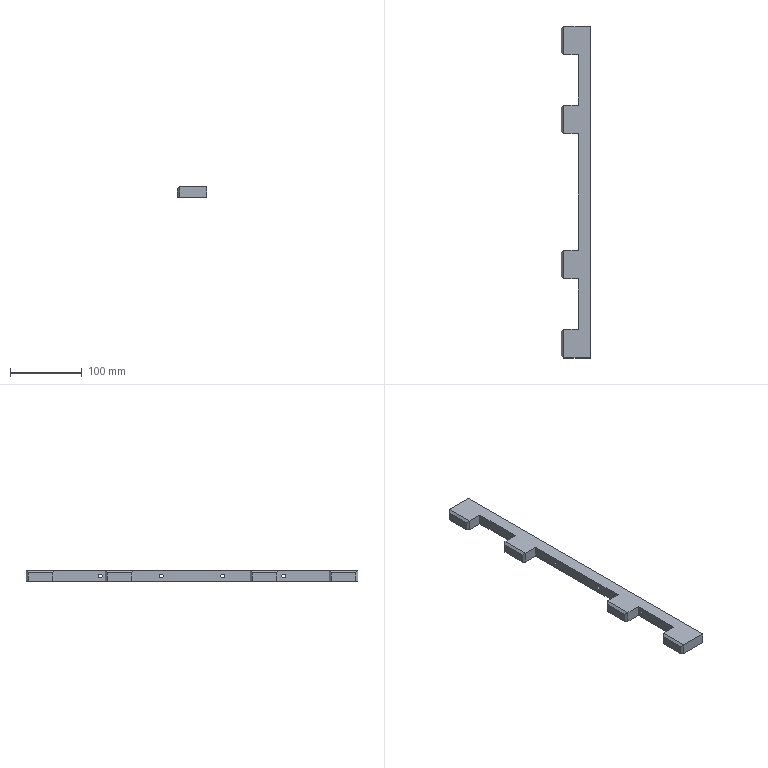Part | SolidWorks | features Chamfer 1, Extrusion 1, HoleWzd 1 | 1 solid | 46 faces | box 40.5 x 462 x 15 mm | volume 171000 mm3 | plane 30 | cylinder 12 | cone 4 | commonest cylinder face diameters 5 x12
STEP:
#1=CARTESIAN_POINT('',(23.5,443.5,10.));
#2=VERTEX_POINT('',#1);
#3=CARTESIAN_POINT('',(23.5,443.5,5.));
#4=VERTEX_POINT('',#3);
#5=CARTESIAN_POINT('',(23.5,443.5,7.5));
#6=DIRECTION('',(1.,0.,0.));
#7=DIRECTION('',(0.,0.,-1.));
#8=AXIS2_PLACEMENT_3D('',#5,#6,#7);
#9=CIRCLE('',#8,2.5);
#10=EDGE_CURVE('',#2,#4,#9,.T.);
#11=ORIENTED_EDGE('',*,*,#10,.F.);
#12=CARTESIAN_POINT('',(40.5,443.5,10.));
#13=VERTEX_POINT('',#12);
#14=CARTESIAN_POINT('',(40.5,443.5,10.));
#15=DIRECTION('',(1.,0.,0.));
#16=VECTOR('',#15,1000.);
#17=LINE('',#14,#16);
#18=EDGE_CURVE('',#2,#13,#17,.T.);
#19=ORIENTED_EDGE('',*,*,#18,.T.);
#20=CARTESIAN_POINT('',(40.5,443.5,5.));
#21=VERTEX_POINT('',#20);
#22=CARTESIAN_POINT('',(40.5,443.5,7.5));
#23=DIRECTION('',(1.,0.,0.));
#24=DIRECTION('',(0.,0.,-1.));
#25=AXIS2_PLACEMENT_3D('',#22,#23,#24);
#26=CIRCLE('',#25,2.5);
#27=EDGE_CURVE('',#13,#21,#26,.T.);
#28=ORIENTED_EDGE('',*,*,#27,.T.);
#29=CARTESIAN_POINT('',(40.5,443.5,5.));
#30=DIRECTION('',(1.,0.,0.));
#31=VECTOR('',#30,1000.);
#32=LINE('',#29,#31);
#33=EDGE_CURVE('',#4,#21,#32,.T.);
#34=ORIENTED_EDGE('',*,*,#33,.F.);
#35=EDGE_LOOP('',(#11,#19,#28,#34));
#36=FACE_OUTER_BOUND('',#35,.T.);
#37=CARTESIAN_POINT('',(40.5,443.5,7.5));
#38=DIRECTION('',(1.,0.,0.));
#39=DIRECTION('',(0.,0.,-1.));
#40=AXIS2_PLACEMENT_3D('',#37,#38,#39);
#41=CYLINDRICAL_SURFACE('',#40,2.5);
#42=ADVANCED_FACE('',(#36),#41,.F.);
#43=CARTESIAN_POINT('',(21.998,443.5,7.5));
#44=VERTEX_POINT('',#43);
#45=CARTESIAN_POINT('',(23.5,443.5,5.));
#46=DIRECTION('',(0.515,0.,-0.8572));
#47=VECTOR('',#46,1000.);
#48=LINE('',#45,#47);
#49=EDGE_CURVE('',#44,#4,#48,.T.);
#50=ORIENTED_EDGE('',*,*,#49,.F.);
#51=CARTESIAN_POINT('',(23.5,443.5,10.));
#52=DIRECTION('',(0.515,0.,0.8572));
#53=VECTOR('',#52,1000.);
#54=LINE('',#51,#53);
#55=EDGE_CURVE('',#44,#2,#54,.T.);
#56=ORIENTED_EDGE('',*,*,#55,.T.);
#57=ORIENTED_EDGE('',*,*,#10,.T.);
#58=EDGE_LOOP('',(#50,#56,#57));
#59=FACE_OUTER_BOUND('',#58,.T.);
#60=CARTESIAN_POINT('',(23.5,443.5,7.5));
#61=DIRECTION('',(1.,0.,0.));
#62=DIRECTION('',(0.,0.,-1.));
#63=AXIS2_PLACEMENT_3D('',#60,#61,#62);
#64=CONICAL_SURFACE('',#63,2.5,1.03);
#65=ADVANCED_FACE('',(#59),#64,.F.);
#66=CARTESIAN_POINT('',(23.5,358.5,10.));
#67=VERTEX_POINT('',#66);
#68=CARTESIAN_POINT('',(23.5,358.5,5.));
#69=VERTEX_POINT('',#68);
#70=CARTESIAN_POINT('',(23.5,358.5,7.5));
#71=DIRECTION('',(1.,0.,0.));
#72=DIRECTION('',(0.,0.,-1.));
#73=AXIS2_PLACEMENT_3D('',#70,#71,#72);
#74=CIRCLE('',#73,2.5);
#75=EDGE_CURVE('',#67,#69,#74,.T.);
#76=ORIENTED_EDGE('',*,*,#75,.F.);
#77=CARTESIAN_POINT('',(40.5,358.5,10.));
#78=VERTEX_POINT('',#77);
#79=CARTESIAN_POINT('',(40.5,358.5,10.));
#80=DIRECTION('',(1.,0.,0.));
#81=VECTOR('',#80,1000.);
#82=LINE('',#79,#81);
#83=EDGE_CURVE('',#67,#78,#82,.T.);
#84=ORIENTED_EDGE('',*,*,#83,.T.);
#85=CARTESIAN_POINT('',(40.5,358.5,5.));
#86=VERTEX_POINT('',#85);
#87=CARTESIAN_POINT('',(40.5,358.5,7.5));
#88=DIRECTION('',(1.,0.,0.));
#89=DIRECTION('',(0.,0.,-1.));
#90=AXIS2_PLACEMENT_3D('',#87,#88,#89);
#91=CIRCLE('',#90,2.5);
#92=EDGE_CURVE('',#78,#86,#91,.T.);
#93=ORIENTED_EDGE('',*,*,#92,.T.);
#94=CARTESIAN_POINT('',(40.5,358.5,5.));
#95=DIRECTION('',(1.,0.,0.));
#96=VECTOR('',#95,1000.);
#97=LINE('',#94,#96);
#98=EDGE_CURVE('',#69,#86,#97,.T.);
#99=ORIENTED_EDGE('',*,*,#98,.F.);
#100=EDGE_LOOP('',(#76,#84,#93,#99));
#101=FACE_OUTER_BOUND('',#100,.T.);
#102=CARTESIAN_POINT('',(40.5,358.5,7.5));
#103=DIRECTION('',(1.,0.,0.));
#104=DIRECTION('',(0.,0.,-1.));
#105=AXIS2_PLACEMENT_3D('',#102,#103,#104);
#106=CYLINDRICAL_SURFACE('',#105,2.5);
#107=ADVANCED_FACE('',(#101),#106,.F.);
#108=CARTESIAN_POINT('',(23.5,273.5,10.));
#109=VERTEX_POINT('',#108);
#110=CARTESIAN_POINT('',(23.5,273.5,5.));
#111=VERTEX_POINT('',#110);
#112=CARTESIAN_POINT('',(23.5,273.5,7.5));
#113=DIRECTION('',(1.,0.,0.));
#114=DIRECTION('',(0.,0.,-1.));
#115=AXIS2_PLACEMENT_3D('',#112,#113,#114);
#116=CIRCLE('',#115,2.5);
#117=EDGE_CURVE('',#109,#111,#116,.T.);
#118=ORIENTED_EDGE('',*,*,#117,.F.);
#119=CARTESIAN_POINT('',(40.5,273.5,10.));
#120=VERTEX_POINT('',#119);
#121=CARTESIAN_POINT('',(40.5,273.5,10.));
#122=DIRECTION('',(1.,0.,0.));
#123=VECTOR('',#122,1000.);
#124=LINE('',#121,#123);
#125=EDGE_CURVE('',#109,#120,#124,.T.);
#126=ORIENTED_EDGE('',*,*,#125,.T.);
#127=CARTESIAN_POINT('',(40.5,273.5,5.));
#128=VERTEX_POINT('',#127);
#129=CARTESIAN_POINT('',(40.5,273.5,7.5));
#130=DIRECTION('',(1.,0.,0.));
#131=DIRECTION('',(0.,0.,-1.));
#132=AXIS2_PLACEMENT_3D('',#129,#130,#131);
#133=CIRCLE('',#132,2.5);
#134=EDGE_CURVE('',#120,#128,#133,.T.);
#135=ORIENTED_EDGE('',*,*,#134,.T.);
#136=CARTESIAN_POINT('',(40.5,273.5,5.));
#137=DIRECTION('',(1.,0.,0.));
#138=VECTOR('',#137,1000.);
#139=LINE('',#136,#138);
#140=EDGE_CURVE('',#111,#128,#139,.T.);
#141=ORIENTED_EDGE('',*,*,#140,.F.);
#142=EDGE_LOOP('',(#118,#126,#135,#141));
#143=FACE_OUTER_BOUND('',#142,.T.);
#144=CARTESIAN_POINT('',(40.5,273.5,7.5));
#145=DIRECTION('',(1.,0.,0.));
#146=DIRECTION('',(0.,0.,-1.));
#147=AXIS2_PLACEMENT_3D('',#144,#145,#146);
#148=CYLINDRICAL_SURFACE('',#147,2.5);
#149=ADVANCED_FACE('',(#143),#148,.F.);
#150=CARTESIAN_POINT('',(23.5,188.5,10.));
#151=VERTEX_POINT('',#150);
#152=CARTESIAN_POINT('',(23.5,188.5,5.));
#153=VERTEX_POINT('',#152);
#154=CARTESIAN_POINT('',(23.5,188.5,7.5));
#155=DIRECTION('',(1.,0.,0.));
#156=DIRECTION('',(0.,0.,-1.));
#157=AXIS2_PLACEMENT_3D('',#154,#155,#156);
#158=CIRCLE('',#157,2.5);
#159=EDGE_CURVE('',#151,#153,#158,.T.);
#160=ORIENTED_EDGE('',*,*,#159,.F.);
#161=CARTESIAN_POINT('',(40.5,188.5,10.));
#162=VERTEX_POINT('',#161);
#163=CARTESIAN_POINT('',(40.5,188.5,10.));
#164=DIRECTION('',(1.,0.,0.));
#165=VECTOR('',#164,1000.);
#166=LINE('',#163,#165);
#167=EDGE_CURVE('',#151,#162,#166,.T.);
#168=ORIENTED_EDGE('',*,*,#167,.T.);
#169=CARTESIAN_POINT('',(40.5,188.5,5.));
#170=VERTEX_POINT('',#169);
#171=CARTESIAN_POINT('',(40.5,188.5,7.5));
#172=DIRECTION('',(1.,0.,0.));
#173=DIRECTION('',(0.,0.,-1.));
#174=AXIS2_PLACEMENT_3D('',#171,#172,#173);
#175=CIRCLE('',#174,2.5);
#176=EDGE_CURVE('',#162,#170,#175,.T.);
#177=ORIENTED_EDGE('',*,*,#176,.T.);
#178=CARTESIAN_POINT('',(40.5,188.5,5.));
#179=DIRECTION('',(1.,0.,0.));
#180=VECTOR('',#179,1000.);
#181=LINE('',#178,#180);
#182=EDGE_CURVE('',#153,#170,#181,.T.);
#183=ORIENTED_EDGE('',*,*,#182,.F.);
#184=EDGE_LOOP('',(#160,#168,#177,#183));
#185=FACE_OUTER_BOUND('',#184,.T.);
#186=CARTESIAN_POINT('',(40.5,188.5,7.5));
#187=DIRECTION('',(1.,0.,0.));
#188=DIRECTION('',(0.,0.,-1.));
#189=AXIS2_PLACEMENT_3D('',#186,#187,#188);
#190=CYLINDRICAL_SURFACE('',#189,2.5);
#191=ADVANCED_FACE('',(#185),#190,.F.);
#192=CARTESIAN_POINT('',(23.5,103.5,10.));
#193=VERTEX_POINT('',#192);
#194=CARTESIAN_POINT('',(23.5,103.5,5.));
#195=VERTEX_POINT('',#194);
#196=CARTESIAN_POINT('',(23.5,103.5,7.5));
#197=DIRECTION('',(1.,0.,0.));
#198=DIRECTION('',(0.,0.,-1.));
#199=AXIS2_PLACEMENT_3D('',#196,#197,#198);
#200=CIRCLE('',#199,2.5);
#201=EDGE_CURVE('',#193,#195,#200,.T.);
#202=ORIENTED_EDGE('',*,*,#201,.F.);
#203=CARTESIAN_POINT('',(40.5,103.5,10.));
#204=VERTEX_POINT('',#203);
#205=CARTESIAN_POINT('',(40.5,103.5,10.));
#206=DIRECTION('',(1.,0.,0.));
#207=VECTOR('',#206,1000.);
#208=LINE('',#205,#207);
#209=EDGE_CURVE('',#193,#204,#208,.T.);
#210=ORIENTED_EDGE('',*,*,#209,.T.);
#211=CARTESIAN_POINT('',(40.5,103.5,5.));
#212=VERTEX_POINT('',#211);
#213=CARTESIAN_POINT('',(40.5,103.5,7.5));
#214=DIRECTION('',(1.,0.,0.));
#215=DIRECTION('',(0.,0.,-1.));
#216=AXIS2_PLACEMENT_3D('',#213,#214,#215);
#217=CIRCLE('',#216,2.5);
#218=EDGE_CURVE('',#204,#212,#217,.T.);
#219=ORIENTED_EDGE('',*,*,#218,.T.);
#220=CARTESIAN_POINT('',(40.5,103.5,5.));
#221=DIRECTION('',(1.,0.,0.));
#222=VECTOR('',#221,1000.);
#223=LINE('',#220,#222);
#224=EDGE_CURVE('',#195,#212,#223,.T.);
#225=ORIENTED_EDGE('',*,*,#224,.F.);
#226=EDGE_LOOP('',(#202,#210,#219,#225));
#227=FACE_OUTER_BOUND('',#226,.T.);
#228=CARTESIAN_POINT('',(40.5,103.5,7.5));
#229=DIRECTION('',(1.,0.,0.));
#230=DIRECTION('',(0.,0.,-1.));
#231=AXIS2_PLACEMENT_3D('',#228,#229,#230);
#232=CYLINDRICAL_SURFACE('',#231,2.5);
#233=ADVANCED_FACE('',(#227),#232,.F.);
#234=CARTESIAN_POINT('',(23.5,18.5,10.));
#235=VERTEX_POINT('',#234);
#236=CARTESIAN_POINT('',(23.5,18.5,5.));
#237=VERTEX_POINT('',#236);
#238=CARTESIAN_POINT('',(23.5,18.5,7.5));
#239=DIRECTION('',(1.,0.,0.));
#240=DIRECTION('',(0.,0.,-1.));
#241=AXIS2_PLACEMENT_3D('',#238,#239,#240);
#242=CIRCLE('',#241,2.5);
#243=EDGE_CURVE('',#235,#237,#242,.T.);
#244=ORIENTED_EDGE('',*,*,#243,.F.);
#245=CARTESIAN_POINT('',(40.5,18.5,10.));
#246=VERTEX_POINT('',#245);
#247=CARTESIAN_POINT('',(40.5,18.5,10.));
#248=DIRECTION('',(1.,0.,0.));
#249=VECTOR('',#248,1000.);
#250=LINE('',#247,#249);
#251=EDGE_CURVE('',#235,#246,#250,.T.);
#252=ORIENTED_EDGE('',*,*,#251,.T.);
#253=CARTESIAN_POINT('',(40.5,18.5,5.));
#254=VERTEX_POINT('',#253);
#255=CARTESIAN_POINT('',(40.5,18.5,7.5));
#256=DIRECTION('',(1.,0.,0.));
#257=DIRECTION('',(0.,0.,-1.));
#258=AXIS2_PLACEMENT_3D('',#255,#256,#257);
#259=CIRCLE('',#258,2.5);
#260=EDGE_CURVE('',#246,#254,#259,.T.);
#261=ORIENTED_EDGE('',*,*,#260,.T.);
#262=CARTESIAN_POINT('',(40.5,18.5,5.));
#263=DIRECTION('',(1.,0.,0.));
#264=VECTOR('',#263,1000.);
#265=LINE('',#262,#264);
#266=EDGE_CURVE('',#237,#254,#265,.T.);
#267=ORIENTED_EDGE('',*,*,#266,.F.);
#268=EDGE_LOOP('',(#244,#252,#261,#267));
#269=FACE_OUTER_BOUND('',#268,.T.);
#270=CARTESIAN_POINT('',(40.5,18.5,7.5));
#271=DIRECTION('',(1.,0.,0.));
#272=DIRECTION('',(0.,0.,-1.));
#273=AXIS2_PLACEMENT_3D('',#270,#271,#272);
#274=CYLINDRICAL_SURFACE('',#273,2.5);
#275=ADVANCED_FACE('',(#269),#274,.F.);
#276=CARTESIAN_POINT('',(21.998,18.5,7.5));
#277=VERTEX_POINT('',#276);
#278=CARTESIAN_POINT('',(23.5,18.5,5.));
#279=DIRECTION('',(0.515,0.,-0.8572));
#280=VECTOR('',#279,1000.);
#281=LINE('',#278,#280);
#282=EDGE_CURVE('',#277,#237,#281,.T.);
#283=ORIENTED_EDGE('',*,*,#282,.F.);
#284=CARTESIAN_POINT('',(23.5,18.5,10.));
#285=DIRECTION('',(0.515,0.,0.8572));
#286=VECTOR('',#285,1000.);
#287=LINE('',#284,#286);
#288=EDGE_CURVE('',#277,#235,#287,.T.);
#289=ORIENTED_EDGE('',*,*,#288,.T.);
#290=ORIENTED_EDGE('',*,*,#243,.T.);
#291=EDGE_LOOP('',(#283,#289,#290));
#292=FACE_OUTER_BOUND('',#291,.T.);
#293=CARTESIAN_POINT('',(23.5,18.5,7.5));
#294=DIRECTION('',(1.,0.,0.));
#295=DIRECTION('',(0.,0.,-1.));
#296=AXIS2_PLACEMENT_3D('',#293,#294,#295);
#297=CONICAL_SURFACE('',#296,2.5,1.03);
#298=ADVANCED_FACE('',(#292),#297,.F.);
#299=CARTESIAN_POINT('',(23.5,103.5,7.5));
#300=DIRECTION('',(1.,0.,0.));
#301=DIRECTION('',(0.,0.,-1.));
#302=AXIS2_PLACEMENT_3D('',#299,#300,#301);
#303=CIRCLE('',#302,2.5);
#304=EDGE_CURVE('',#195,#193,#303,.T.);
#305=ORIENTED_EDGE('',*,*,#304,.T.);
#306=ORIENTED_EDGE('',*,*,#201,.T.);
#307=EDGE_LOOP('',(#305,#306));
#308=FACE_BOUND('',#307,.T.);
#309=CARTESIAN_POINT('',(23.5,40.,0.));
#310=VERTEX_POINT('',#309);
#311=CARTESIAN_POINT('',(23.5,110.,0.));
#312=VERTEX_POINT('',#311);
#313=CARTESIAN_POINT('',(23.5,0.,0.));
#314=DIRECTION('',(0.,1.,0.));
#315=VECTOR('',#314,1000.);
#316=LINE('',#313,#315);
#317=EDGE_CURVE('',#310,#312,#316,.T.);
#318=ORIENTED_EDGE('',*,*,#317,.F.);
#319=CARTESIAN_POINT('',(23.5,40.,15.));
#320=VERTEX_POINT('',#319);
#321=CARTESIAN_POINT('',(23.5,40.,15.));
#322=DIRECTION('',(0.,0.,-1.));
#323=VECTOR('',#322,1000.);
#324=LINE('',#321,#323);
#325=EDGE_CURVE('',#320,#310,#324,.T.);
#326=ORIENTED_EDGE('',*,*,#325,.F.);
#327=CARTESIAN_POINT('',(23.5,110.,15.));
#328=VERTEX_POINT('',#327);
#329=CARTESIAN_POINT('',(23.5,0.,15.));
#330=DIRECTION('',(0.,1.,0.));
#331=VECTOR('',#330,1000.);
#332=LINE('',#329,#331);
#333=EDGE_CURVE('',#320,#328,#332,.T.);
#334=ORIENTED_EDGE('',*,*,#333,.T.);
#335=CARTESIAN_POINT('',(23.5,110.,15.));
#336=DIRECTION('',(0.,0.,-1.));
#337=VECTOR('',#336,1000.);
#338=LINE('',#335,#337);
#339=EDGE_CURVE('',#328,#312,#338,.T.);
#340=ORIENTED_EDGE('',*,*,#339,.T.);
#341=EDGE_LOOP('',(#318,#326,#334,#340));
#342=FACE_OUTER_BOUND('',#341,.T.);
#343=CARTESIAN_POINT('',(23.5,0.,15.));
#344=DIRECTION('',(-1.,0.,0.));
#345=DIRECTION('',(0.,0.,1.));
#346=AXIS2_PLACEMENT_3D('',#343,#344,#345);
#347=PLANE('',#346);
#348=ADVANCED_FACE('',(#308,#342),#347,.T.);
#349=CARTESIAN_POINT('',(3.,40.,0.));
#350=VERTEX_POINT('',#349);
#351=CARTESIAN_POINT('',(0.,40.,0.));
#352=DIRECTION('',(1.,0.,0.));
#353=VECTOR('',#352,1000.);
#354=LINE('',#351,#353);
#355=EDGE_CURVE('',#350,#310,#354,.T.);
#356=ORIENTED_EDGE('',*,*,#355,.F.);
#357=CARTESIAN_POINT('',(3.,40.,15.));
#358=VERTEX_POINT('',#357);
#359=CARTESIAN_POINT('',(3.,40.,15.));
#360=DIRECTION('',(0.,0.,1.));
#361=VECTOR('',#360,1000.);
#362=LINE('',#359,#361);
#363=EDGE_CURVE('',#350,#358,#362,.T.);
#364=ORIENTED_EDGE('',*,*,#363,.T.);
#365=CARTESIAN_POINT('',(0.,40.,15.));
#366=DIRECTION('',(1.,0.,0.));
#367=VECTOR('',#366,1000.);
#368=LINE('',#365,#367);
#369=EDGE_CURVE('',#358,#320,#368,.T.);
#370=ORIENTED_EDGE('',*,*,#369,.T.);
#371=ORIENTED_EDGE('',*,*,#325,.T.);
#372=EDGE_LOOP('',(#356,#364,#370,#371));
#373=FACE_OUTER_BOUND('',#372,.T.);
#374=CARTESIAN_POINT('',(0.,40.,15.));
#375=DIRECTION('',(0.,1.,0.));
#376=DIRECTION('',(-1.,0.,0.));
#377=AXIS2_PLACEMENT_3D('',#374,#375,#376);
#378=PLANE('',#377);
#379=ADVANCED_FACE('',(#373),#378,.T.);
#380=CARTESIAN_POINT('',(0.,37.,0.));
#381=VERTEX_POINT('',#380);
#382=CARTESIAN_POINT('',(0.,3.,0.));
#383=VERTEX_POINT('',#382);
#384=CARTESIAN_POINT('',(0.,0.,0.));
#385=DIRECTION('',(0.,-1.,0.));
#386=VECTOR('',#385,1000.);
#387=LINE('',#384,#386);
#388=EDGE_CURVE('',#381,#383,#387,.T.);
#389=ORIENTED_EDGE('',*,*,#388,.T.);
#390=CARTESIAN_POINT('',(0.,3.,12.));
#391=VERTEX_POINT('',#390);
#392=CARTESIAN_POINT('',(0.,3.,15.));
#393=DIRECTION('',(0.,0.,1.));
#394=VECTOR('',#393,1000.);
#395=LINE('',#392,#394);
#396=EDGE_CURVE('',#383,#391,#395,.T.);
#397=ORIENTED_EDGE('',*,*,#396,.T.);
#398=CARTESIAN_POINT('',(0.,37.,12.));
#399=VERTEX_POINT('',#398);
#400=CARTESIAN_POINT('',(0.,40.,12.));
#401=DIRECTION('',(0.,1.,0.));
#402=VECTOR('',#401,1000.);
#403=LINE('',#400,#402);
#404=EDGE_CURVE('',#391,#399,#403,.T.);
#405=ORIENTED_EDGE('',*,*,#404,.T.);
#406=CARTESIAN_POINT('',(0.,37.,0.));
#407=DIRECTION('',(0.,0.,-1.));
#408=VECTOR('',#407,1000.);
#409=LINE('',#406,#408);
#410=EDGE_CURVE('',#399,#381,#409,.T.);
#411=ORIENTED_EDGE('',*,*,#410,.T.);
#412=EDGE_LOOP('',(#389,#397,#405,#411));
#413=FACE_OUTER_BOUND('',#412,.T.);
#414=CARTESIAN_POINT('',(0.,0.,15.));
#415=DIRECTION('',(1.,0.,0.));
#416=DIRECTION('',(0.,0.,-1.));
#417=AXIS2_PLACEMENT_3D('',#414,#415,#416);
#418=PLANE('',#417);
#419=ADVANCED_FACE('',(#413),#418,.F.);
#420=CARTESIAN_POINT('',(3.,0.,15.));
#421=VERTEX_POINT('',#420);
#422=CARTESIAN_POINT('',(40.5,0.,15.));
#423=VERTEX_POINT('',#422);
#424=CARTESIAN_POINT('',(0.,0.,15.));
#425=DIRECTION('',(1.,0.,0.));
#426=VECTOR('',#425,1000.);
#427=LINE('',#424,#426);
#428=EDGE_CURVE('',#421,#423,#427,.T.);
#429=ORIENTED_EDGE('',*,*,#428,.F.);
#430=CARTESIAN_POINT('',(3.,0.,0.));
#431=VERTEX_POINT('',#430);
#432=CARTESIAN_POINT('',(3.,0.,15.));
#433=DIRECTION('',(0.,0.,-1.));
#434=VECTOR('',#433,1000.);
#435=LINE('',#432,#434);
#436=EDGE_CURVE('',#421,#431,#435,.T.);
#437=ORIENTED_EDGE('',*,*,#436,.T.);
#438=CARTESIAN_POINT('',(40.5,0.,0.));
#439=VERTEX_POINT('',#438);
#440=CARTESIAN_POINT('',(0.,0.,0.));
#441=DIRECTION('',(1.,0.,0.));
#442=VECTOR('',#441,1000.);
#443=LINE('',#440,#442);
#444=EDGE_CURVE('',#431,#439,#443,.T.);
#445=ORIENTED_EDGE('',*,*,#444,.T.);
#446=CARTESIAN_POINT('',(40.5,0.,15.));
#447=DIRECTION('',(0.,0.,-1.));
#448=VECTOR('',#447,1000.);
#449=LINE('',#446,#448);
#450=EDGE_CURVE('',#423,#439,#449,.T.);
#451=ORIENTED_EDGE('',*,*,#450,.F.);
#452=EDGE_LOOP('',(#429,#437,#445,#451));
#453=FACE_OUTER_BOUND('',#452,.T.);
#454=CARTESIAN_POINT('',(0.,0.,15.));
#455=DIRECTION('',(0.,1.,0.));
#456=DIRECTION('',(0.,0.,1.));
#457=AXIS2_PLACEMENT_3D('',#454,#455,#456);
#458=PLANE('',#457);
#459=ADVANCED_FACE('',(#453),#458,.F.);
#460=CARTESIAN_POINT('',(40.5,443.5,7.5));
#461=DIRECTION('',(1.,0.,0.));
#462=DIRECTION('',(0.,0.,-1.));
#463=AXIS2_PLACEMENT_3D('',#460,#461,#462);
#464=CIRCLE('',#463,2.5);
#465=EDGE_CURVE('',#21,#13,#464,.T.);
#466=ORIENTED_EDGE('',*,*,#465,.F.);
#467=ORIENTED_EDGE('',*,*,#27,.F.);
#468=EDGE_LOOP('',(#466,#467));
#469=FACE_BOUND('',#468,.T.);
#470=CARTESIAN_POINT('',(40.5,358.5,7.5));
#471=DIRECTION('',(1.,0.,0.));
#472=DIRECTION('',(0.,0.,-1.));
#473=AXIS2_PLACEMENT_3D('',#470,#471,#472);
#474=CIRCLE('',#473,2.5);
#475=EDGE_CURVE('',#86,#78,#474,.T.);
#476=ORIENTED_EDGE('',*,*,#475,.F.);
#477=ORIENTED_EDGE('',*,*,#92,.F.);
#478=EDGE_LOOP('',(#476,#477));
#479=FACE_BOUND('',#478,.T.);
#480=CARTESIAN_POINT('',(40.5,273.5,7.5));
#481=DIRECTION('',(1.,0.,0.));
#482=DIRECTION('',(0.,0.,-1.));
#483=AXIS2_PLACEMENT_3D('',#480,#481,#482);
#484=CIRCLE('',#483,2.5);
#485=EDGE_CURVE('',#128,#120,#484,.T.);
#486=ORIENTED_EDGE('',*,*,#485,.F.);
#487=ORIENTED_EDGE('',*,*,#134,.F.);
#488=EDGE_LOOP('',(#486,#487));
#489=FACE_BOUND('',#488,.T.);
#490=CARTESIAN_POINT('',(40.5,188.5,7.5));
#491=DIRECTION('',(1.,0.,0.));
#492=DIRECTION('',(0.,0.,-1.));
#493=AXIS2_PLACEMENT_3D('',#490,#491,#492);
#494=CIRCLE('',#493,2.5);
#495=EDGE_CURVE('',#170,#162,#494,.T.);
#496=ORIENTED_EDGE('',*,*,#495,.F.);
#497=ORIENTED_EDGE('',*,*,#176,.F.);
#498=EDGE_LOOP('',(#496,#497));
#499=FACE_BOUND('',#498,.T.);
#500=CARTESIAN_POINT('',(40.5,103.5,7.5));
#501=DIRECTION('',(1.,0.,0.));
#502=DIRECTION('',(0.,0.,-1.));
#503=AXIS2_PLACEMENT_3D('',#500,#501,#502);
#504=CIRCLE('',#503,2.5);
#505=EDGE_CURVE('',#212,#204,#504,.T.);
#506=ORIENTED_EDGE('',*,*,#505,.F.);
#507=ORIENTED_EDGE('',*,*,#218,.F.);
#508=EDGE_LOOP('',(#506,#507));
#509=FACE_BOUND('',#508,.T.);
#510=CARTESIAN_POINT('',(40.5,18.5,7.5));
#511=DIRECTION('',(1.,0.,0.));
#512=DIRECTION('',(0.,0.,-1.));
#513=AXIS2_PLACEMENT_3D('',#510,#511,#512);
#514=CIRCLE('',#513,2.5);
#515=EDGE_CURVE('',#254,#246,#514,.T.);
#516=ORIENTED_EDGE('',*,*,#515,.F.);
#517=ORIENTED_EDGE('',*,*,#260,.F.);
#518=EDGE_LOOP('',(#516,#517));
#519=FACE_BOUND('',#518,.T.);
#520=CARTESIAN_POINT('',(40.5,462.,0.));
#521=VERTEX_POINT('',#520);
#522=CARTESIAN_POINT('',(40.5,0.,0.));
#523=DIRECTION('',(0.,-1.,0.));
#524=VECTOR('',#523,1000.);
#525=LINE('',#522,#524);
#526=EDGE_CURVE('',#521,#439,#525,.T.);
#527=ORIENTED_EDGE('',*,*,#526,.F.);
#528=CARTESIAN_POINT('',(40.5,462.,15.));
#529=VERTEX_POINT('',#528);
#530=CARTESIAN_POINT('',(40.5,462.,15.));
#531=DIRECTION('',(0.,0.,-1.));
#532=VECTOR('',#531,1000.);
#533=LINE('',#530,#532);
#534=EDGE_CURVE('',#529,#521,#533,.T.);
#535=ORIENTED_EDGE('',*,*,#534,.F.);
#536=CARTESIAN_POINT('',(40.5,0.,15.));
#537=DIRECTION('',(0.,-1.,0.));
#538=VECTOR('',#537,1000.);
#539=LINE('',#536,#538);
#540=EDGE_CURVE('',#529,#423,#539,.T.);
#541=ORIENTED_EDGE('',*,*,#540,.T.);
#542=ORIENTED_EDGE('',*,*,#450,.T.);
#543=EDGE_LOOP('',(#527,#535,#541,#542));
#544=FACE_OUTER_BOUND('',#543,.T.);
#545=CARTESIAN_POINT('',(40.5,0.,15.));
#546=DIRECTION('',(1.,0.,0.));
#547=DIRECTION('',(0.,1.,0.));
#548=AXIS2_PLACEMENT_3D('',#545,#546,#547);
#549=PLANE('',#548);
#550=ADVANCED_FACE('',(#469,#479,#489,#499,#509,#519,#544),#549,.T.);
#551=CARTESIAN_POINT('',(3.,462.,0.));
#552=VERTEX_POINT('',#551);
#553=CARTESIAN_POINT('',(0.,462.,0.));
#554=DIRECTION('',(1.,0.,0.));
#555=VECTOR('',#554,1000.);
#556=LINE('',#553,#555);
#557=EDGE_CURVE('',#552,#521,#556,.T.);
#558=ORIENTED_EDGE('',*,*,#557,.F.);
#559=CARTESIAN_POINT('',(3.,462.,15.));
#560=VERTEX_POINT('',#559);
#561=CARTESIAN_POINT('',(3.,462.,15.));
#562=DIRECTION('',(0.,0.,1.));
#563=VECTOR('',#562,1000.);
#564=LINE('',#561,#563);
#565=EDGE_CURVE('',#552,#560,#564,.T.);
#566=ORIENTED_EDGE('',*,*,#565,.T.);
#567=CARTESIAN_POINT('',(0.,462.,15.));
#568=DIRECTION('',(1.,0.,0.));
#569=VECTOR('',#568,1000.);
#570=LINE('',#567,#569);
#571=EDGE_CURVE('',#560,#529,#570,.T.);
#572=ORIENTED_EDGE('',*,*,#571,.T.);
#573=ORIENTED_EDGE('',*,*,#534,.T.);
#574=EDGE_LOOP('',(#558,#566,#572,#573));
#575=FACE_OUTER_BOUND('',#574,.T.);
#576=CARTESIAN_POINT('',(0.,462.,15.));
#577=DIRECTION('',(0.,1.,0.));
#578=DIRECTION('',(0.,0.,1.));
#579=AXIS2_PLACEMENT_3D('',#576,#577,#578);
#580=PLANE('',#579);
#581=ADVANCED_FACE('',(#575),#580,.T.);
#582=CARTESIAN_POINT('',(0.,459.,0.));
#583=VERTEX_POINT('',#582);
#584=CARTESIAN_POINT('',(0.,425.,0.));
#585=VERTEX_POINT('',#584);
#586=CARTESIAN_POINT('',(0.,0.,0.));
#587=DIRECTION('',(0.,-1.,0.));
#588=VECTOR('',#587,1000.);
#589=LINE('',#586,#588);
#590=EDGE_CURVE('',#583,#585,#589,.T.);
#591=ORIENTED_EDGE('',*,*,#590,.T.);
#592=CARTESIAN_POINT('',(0.,425.,12.));
#593=VERTEX_POINT('',#592);
#594=CARTESIAN_POINT('',(0.,425.,15.));
#595=DIRECTION('',(0.,0.,1.));
#596=VECTOR('',#595,1000.);
#597=LINE('',#594,#596);
#598=EDGE_CURVE('',#585,#593,#597,.T.);
#599=ORIENTED_EDGE('',*,*,#598,.T.);
#600=CARTESIAN_POINT('',(0.,459.,12.));
#601=VERTEX_POINT('',#600);
#602=CARTESIAN_POINT('',(0.,462.,12.));
#603=DIRECTION('',(0.,1.,0.));
#604=VECTOR('',#603,1000.);
#605=LINE('',#602,#604);
#606=EDGE_CURVE('',#593,#601,#605,.T.);
#607=ORIENTED_EDGE('',*,*,#606,.T.);
#608=CARTESIAN_POINT('',(0.,459.,0.));
#609=DIRECTION('',(0.,0.,-1.));
#610=VECTOR('',#609,1000.);
#611=LINE('',#608,#610);
#612=EDGE_CURVE('',#601,#583,#611,.T.);
#613=ORIENTED_EDGE('',*,*,#612,.T.);
#614=EDGE_LOOP('',(#591,#599,#607,#613));
#615=FACE_OUTER_BOUND('',#614,.T.);
#616=CARTESIAN_POINT('',(0.,0.,15.));
#617=DIRECTION('',(1.,0.,0.));
#618=DIRECTION('',(0.,0.,-1.));
#619=AXIS2_PLACEMENT_3D('',#616,#617,#618);
#620=PLANE('',#619);
#621=ADVANCED_FACE('',(#615),#620,.F.);
#622=CARTESIAN_POINT('',(3.,422.,15.));
#623=VERTEX_POINT('',#622);
#624=CARTESIAN_POINT('',(23.5,422.,15.));
#625=VERTEX_POINT('',#624);
#626=CARTESIAN_POINT('',(0.,422.,15.));
#627=DIRECTION('',(1.,0.,0.));
#628=VECTOR('',#627,1000.);
#629=LINE('',#626,#628);
#630=EDGE_CURVE('',#623,#625,#629,.T.);
#631=ORIENTED_EDGE('',*,*,#630,.F.);
#632=CARTESIAN_POINT('',(3.,422.,0.));
#633=VERTEX_POINT('',#632);
#634=CARTESIAN_POINT('',(3.,422.,15.));
#635=DIRECTION('',(0.,0.,-1.));
#636=VECTOR('',#635,1000.);
#637=LINE('',#634,#636);
#638=EDGE_CURVE('',#623,#633,#637,.T.);
#639=ORIENTED_EDGE('',*,*,#638,.T.);
#640=CARTESIAN_POINT('',(23.5,422.,0.));
#641=VERTEX_POINT('',#640);
#642=CARTESIAN_POINT('',(0.,422.,0.));
#643=DIRECTION('',(1.,0.,0.));
#644=VECTOR('',#643,1000.);
#645=LINE('',#642,#644);
#646=EDGE_CURVE('',#633,#641,#645,.T.);
#647=ORIENTED_EDGE('',*,*,#646,.T.);
#648=CARTESIAN_POINT('',(23.5,422.,15.));
#649=DIRECTION('',(0.,0.,-1.));
#650=VECTOR('',#649,1000.);
#651=LINE('',#648,#650);
#652=EDGE_CURVE('',#625,#641,#651,.T.);
#653=ORIENTED_EDGE('',*,*,#652,.F.);
#654=EDGE_LOOP('',(#631,#639,#647,#653));
#655=FACE_OUTER_BOUND('',#654,.T.);
#656=CARTESIAN_POINT('',(0.,422.,15.));
#657=DIRECTION('',(0.,1.,0.));
#658=DIRECTION('',(0.,0.,1.));
#659=AXIS2_PLACEMENT_3D('',#656,#657,#658);
#660=PLANE('',#659);
#661=ADVANCED_FACE('',(#655),#660,.F.);
#662=CARTESIAN_POINT('',(23.5,358.5,7.5));
#663=DIRECTION('',(1.,0.,0.));
#664=DIRECTION('',(0.,0.,-1.));
#665=AXIS2_PLACEMENT_3D('',#662,#663,#664);
#666=CIRCLE('',#665,2.5);
#667=EDGE_CURVE('',#69,#67,#666,.T.);
#668=ORIENTED_EDGE('',*,*,#667,.T.);
#669=ORIENTED_EDGE('',*,*,#75,.T.);
#670=EDGE_LOOP('',(#668,#669));
#671=FACE_BOUND('',#670,.T.);
#672=CARTESIAN_POINT('',(23.5,352.,0.));
#673=VERTEX_POINT('',#672);
#674=CARTESIAN_POINT('',(23.5,0.,0.));
#675=DIRECTION('',(0.,1.,0.));
#676=VECTOR('',#675,1000.);
#677=LINE('',#674,#676);
#678=EDGE_CURVE('',#673,#641,#677,.T.);
#679=ORIENTED_EDGE('',*,*,#678,.F.);
#680=CARTESIAN_POINT('',(23.5,352.,15.));
#681=VERTEX_POINT('',#680);
#682=CARTESIAN_POINT('',(23.5,352.,15.));
#683=DIRECTION('',(0.,0.,-1.));
#684=VECTOR('',#683,1000.);
#685=LINE('',#682,#684);
#686=EDGE_CURVE('',#681,#673,#685,.T.);
#687=ORIENTED_EDGE('',*,*,#686,.F.);
#688=CARTESIAN_POINT('',(23.5,0.,15.));
#689=DIRECTION('',(0.,1.,0.));
#690=VECTOR('',#689,1000.);
#691=LINE('',#688,#690);
#692=EDGE_CURVE('',#681,#625,#691,.T.);
#693=ORIENTED_EDGE('',*,*,#692,.T.);
#694=ORIENTED_EDGE('',*,*,#652,.T.);
#695=EDGE_LOOP('',(#679,#687,#693,#694));
#696=FACE_OUTER_BOUND('',#695,.T.);
#697=CARTESIAN_POINT('',(23.5,0.,15.));
#698=DIRECTION('',(-1.,0.,0.));
#699=DIRECTION('',(0.,0.,1.));
#700=AXIS2_PLACEMENT_3D('',#697,#698,#699);
#701=PLANE('',#700);
#702=ADVANCED_FACE('',(#671,#696),#701,.T.);
#703=CARTESIAN_POINT('',(3.,352.,0.));
#704=VERTEX_POINT('',#703);
#705=CARTESIAN_POINT('',(0.,352.,0.));
#706=DIRECTION('',(1.,0.,0.));
#707=VECTOR('',#706,1000.);
#708=LINE('',#705,#707);
#709=EDGE_CURVE('',#704,#673,#708,.T.);
#710=ORIENTED_EDGE('',*,*,#709,.F.);
#711=CARTESIAN_POINT('',(3.,352.,15.));
#712=VERTEX_POINT('',#711);
#713=CARTESIAN_POINT('',(3.,352.,15.));
#714=DIRECTION('',(0.,0.,1.));
#715=VECTOR('',#714,1000.);
#716=LINE('',#713,#715);
#717=EDGE_CURVE('',#704,#712,#716,.T.);
#718=ORIENTED_EDGE('',*,*,#717,.T.);
#719=CARTESIAN_POINT('',(0.,352.,15.));
#720=DIRECTION('',(1.,0.,0.));
#721=VECTOR('',#720,1000.);
#722=LINE('',#719,#721);
#723=EDGE_CURVE('',#712,#681,#722,.T.);
#724=ORIENTED_EDGE('',*,*,#723,.T.);
#725=ORIENTED_EDGE('',*,*,#686,.T.);
#726=EDGE_LOOP('',(#710,#718,#724,#725));
#727=FACE_OUTER_BOUND('',#726,.T.);
#728=CARTESIAN_POINT('',(0.,352.,15.));
#729=DIRECTION('',(0.,1.,0.));
#730=DIRECTION('',(0.,0.,1.));
#731=AXIS2_PLACEMENT_3D('',#728,#729,#730);
#732=PLANE('',#731);
#733=ADVANCED_FACE('',(#727),#732,.T.);
#734=CARTESIAN_POINT('',(0.,349.,0.));
#735=VERTEX_POINT('',#734);
#736=CARTESIAN_POINT('',(0.,315.,0.));
#737=VERTEX_POINT('',#736);
#738=CARTESIAN_POINT('',(0.,0.,0.));
#739=DIRECTION('',(0.,-1.,0.));
#740=VECTOR('',#739,1000.);
#741=LINE('',#738,#740);
#742=EDGE_CURVE('',#735,#737,#741,.T.);
#743=ORIENTED_EDGE('',*,*,#742,.T.);
#744=CARTESIAN_POINT('',(0.,315.,12.));
#745=VERTEX_POINT('',#744);
#746=CARTESIAN_POINT('',(0.,315.,15.));
#747=DIRECTION('',(0.,0.,1.));
#748=VECTOR('',#747,1000.);
#749=LINE('',#746,#748);
#750=EDGE_CURVE('',#737,#745,#749,.T.);
#751=ORIENTED_EDGE('',*,*,#750,.T.);
#752=CARTESIAN_POINT('',(0.,349.,12.));
#753=VERTEX_POINT('',#752);
#754=CARTESIAN_POINT('',(0.,352.,12.));
#755=DIRECTION('',(0.,1.,0.));
#756=VECTOR('',#755,1000.);
#757=LINE('',#754,#756);
#758=EDGE_CURVE('',#745,#753,#757,.T.);
#759=ORIENTED_EDGE('',*,*,#758,.T.);
#760=CARTESIAN_POINT('',(0.,349.,0.));
#761=DIRECTION('',(0.,0.,-1.));
#762=VECTOR('',#761,1000.);
#763=LINE('',#760,#762);
#764=EDGE_CURVE('',#753,#735,#763,.T.);
#765=ORIENTED_EDGE('',*,*,#764,.T.);
#766=EDGE_LOOP('',(#743,#751,#759,#765));
#767=FACE_OUTER_BOUND('',#766,.T.);
#768=CARTESIAN_POINT('',(0.,0.,15.));
#769=DIRECTION('',(1.,0.,0.));
#770=DIRECTION('',(0.,0.,-1.));
#771=AXIS2_PLACEMENT_3D('',#768,#769,#770);
#772=PLANE('',#771);
#773=ADVANCED_FACE('',(#767),#772,.F.);
#774=CARTESIAN_POINT('',(3.,312.,15.));
#775=VERTEX_POINT('',#774);
#776=CARTESIAN_POINT('',(23.5,312.,15.));
#777=VERTEX_POINT('',#776);
#778=CARTESIAN_POINT('',(0.,312.,15.));
#779=DIRECTION('',(1.,0.,0.));
#780=VECTOR('',#779,1000.);
#781=LINE('',#778,#780);
#782=EDGE_CURVE('',#775,#777,#781,.T.);
#783=ORIENTED_EDGE('',*,*,#782,.F.);
#784=CARTESIAN_POINT('',(3.,312.,0.));
#785=VERTEX_POINT('',#784);
#786=CARTESIAN_POINT('',(3.,312.,15.));
#787=DIRECTION('',(0.,0.,-1.));
#788=VECTOR('',#787,1000.);
#789=LINE('',#786,#788);
#790=EDGE_CURVE('',#775,#785,#789,.T.);
#791=ORIENTED_EDGE('',*,*,#790,.T.);
#792=CARTESIAN_POINT('',(23.5,312.,0.));
#793=VERTEX_POINT('',#792);
#794=CARTESIAN_POINT('',(0.,312.,0.));
#795=DIRECTION('',(1.,0.,0.));
#796=VECTOR('',#795,1000.);
#797=LINE('',#794,#796);
#798=EDGE_CURVE('',#785,#793,#797,.T.);
#799=ORIENTED_EDGE('',*,*,#798,.T.);
#800=CARTESIAN_POINT('',(23.5,312.,15.));
#801=DIRECTION('',(0.,0.,-1.));
#802=VECTOR('',#801,1000.);
#803=LINE('',#800,#802);
#804=EDGE_CURVE('',#777,#793,#803,.T.);
#805=ORIENTED_EDGE('',*,*,#804,.F.);
#806=EDGE_LOOP('',(#783,#791,#799,#805));
#807=FACE_OUTER_BOUND('',#806,.T.);
#808=CARTESIAN_POINT('',(0.,312.,15.));
#809=DIRECTION('',(0.,1.,0.));
#810=DIRECTION('',(0.,0.,1.));
#811=AXIS2_PLACEMENT_3D('',#808,#809,#810);
#812=PLANE('',#811);
#813=ADVANCED_FACE('',(#807),#812,.F.);
#814=CARTESIAN_POINT('',(23.5,273.5,7.5));
#815=DIRECTION('',(1.,0.,0.));
#816=DIRECTION('',(0.,0.,-1.));
#817=AXIS2_PLACEMENT_3D('',#814,#815,#816);
#818=CIRCLE('',#817,2.5);
#819=EDGE_CURVE('',#111,#109,#818,.T.);
#820=ORIENTED_EDGE('',*,*,#819,.T.);
#821=ORIENTED_EDGE('',*,*,#117,.T.);
#822=EDGE_LOOP('',(#820,#821));
#823=FACE_BOUND('',#822,.T.);
#824=CARTESIAN_POINT('',(23.5,188.5,7.5));
#825=DIRECTION('',(1.,0.,0.));
#826=DIRECTION('',(0.,0.,-1.));
#827=AXIS2_PLACEMENT_3D('',#824,#825,#826);
#828=CIRCLE('',#827,2.5);
#829=EDGE_CURVE('',#153,#151,#828,.T.);
#830=ORIENTED_EDGE('',*,*,#829,.T.);
#831=ORIENTED_EDGE('',*,*,#159,.T.);
#832=EDGE_LOOP('',(#830,#831));
#833=FACE_BOUND('',#832,.T.);
#834=CARTESIAN_POINT('',(23.5,150.,0.));
#835=VERTEX_POINT('',#834);
#836=CARTESIAN_POINT('',(23.5,0.,0.));
#837=DIRECTION('',(0.,1.,0.));
#838=VECTOR('',#837,1000.);
#839=LINE('',#836,#838);
#840=EDGE_CURVE('',#835,#793,#839,.T.);
#841=ORIENTED_EDGE('',*,*,#840,.F.);
#842=CARTESIAN_POINT('',(23.5,150.,15.));
#843=VERTEX_POINT('',#842);
#844=CARTESIAN_POINT('',(23.5,150.,15.));
#845=DIRECTION('',(0.,0.,-1.));
#846=VECTOR('',#845,1000.);
#847=LINE('',#844,#846);
#848=EDGE_CURVE('',#843,#835,#847,.T.);
#849=ORIENTED_EDGE('',*,*,#848,.F.);
#850=CARTESIAN_POINT('',(23.5,0.,15.));
#851=DIRECTION('',(0.,1.,0.));
#852=VECTOR('',#851,1000.);
#853=LINE('',#850,#852);
#854=EDGE_CURVE('',#843,#777,#853,.T.);
#855=ORIENTED_EDGE('',*,*,#854,.T.);
#856=ORIENTED_EDGE('',*,*,#804,.T.);
#857=EDGE_LOOP('',(#841,#849,#855,#856));
#858=FACE_OUTER_BOUND('',#857,.T.);
#859=CARTESIAN_POINT('',(23.5,0.,15.));
#860=DIRECTION('',(-1.,0.,0.));
#861=DIRECTION('',(0.,0.,1.));
#862=AXIS2_PLACEMENT_3D('',#859,#860,#861);
#863=PLANE('',#862);
#864=ADVANCED_FACE('',(#823,#833,#858),#863,.T.);
#865=CARTESIAN_POINT('',(3.,150.,0.));
#866=VERTEX_POINT('',#865);
#867=CARTESIAN_POINT('',(0.,150.,0.));
#868=DIRECTION('',(1.,0.,0.));
#869=VECTOR('',#868,1000.);
#870=LINE('',#867,#869);
#871=EDGE_CURVE('',#866,#835,#870,.T.);
#872=ORIENTED_EDGE('',*,*,#871,.F.);
#873=CARTESIAN_POINT('',(3.,150.,15.));
#874=VERTEX_POINT('',#873);
#875=CARTESIAN_POINT('',(3.,150.,15.));
#876=DIRECTION('',(0.,0.,1.));
#877=VECTOR('',#876,1000.);
#878=LINE('',#875,#877);
#879=EDGE_CURVE('',#866,#874,#878,.T.);
#880=ORIENTED_EDGE('',*,*,#879,.T.);
#881=CARTESIAN_POINT('',(0.,150.,15.));
#882=DIRECTION('',(1.,0.,0.));
#883=VECTOR('',#882,1000.);
#884=LINE('',#881,#883);
#885=EDGE_CURVE('',#874,#843,#884,.T.);
#886=ORIENTED_EDGE('',*,*,#885,.T.);
#887=ORIENTED_EDGE('',*,*,#848,.T.);
#888=EDGE_LOOP('',(#872,#880,#886,#887));
#889=FACE_OUTER_BOUND('',#888,.T.);
#890=CARTESIAN_POINT('',(0.,150.,15.));
#891=DIRECTION('',(0.,1.,0.));
#892=DIRECTION('',(-1.,0.,0.));
#893=AXIS2_PLACEMENT_3D('',#890,#891,#892);
#894=PLANE('',#893);
#895=ADVANCED_FACE('',(#889),#894,.T.);
#896=CARTESIAN_POINT('',(0.,147.,0.));
#897=VERTEX_POINT('',#896);
#898=CARTESIAN_POINT('',(0.,113.,0.));
#899=VERTEX_POINT('',#898);
#900=CARTESIAN_POINT('',(0.,0.,0.));
#901=DIRECTION('',(0.,-1.,0.));
#902=VECTOR('',#901,1000.);
#903=LINE('',#900,#902);
#904=EDGE_CURVE('',#897,#899,#903,.T.);
#905=ORIENTED_EDGE('',*,*,#904,.T.);
#906=CARTESIAN_POINT('',(0.,113.,12.));
#907=VERTEX_POINT('',#906);
#908=CARTESIAN_POINT('',(0.,113.,15.));
#909=DIRECTION('',(0.,0.,1.));
#910=VECTOR('',#909,1000.);
#911=LINE('',#908,#910);
#912=EDGE_CURVE('',#899,#907,#911,.T.);
#913=ORIENTED_EDGE('',*,*,#912,.T.);
#914=CARTESIAN_POINT('',(0.,147.,12.));
#915=VERTEX_POINT('',#914);
#916=CARTESIAN_POINT('',(0.,150.,12.));
#917=DIRECTION('',(0.,1.,0.));
#918=VECTOR('',#917,1000.);
#919=LINE('',#916,#918);
#920=EDGE_CURVE('',#907,#915,#919,.T.);
#921=ORIENTED_EDGE('',*,*,#920,.T.);
#922=CARTESIAN_POINT('',(0.,147.,0.));
#923=DIRECTION('',(0.,0.,-1.));
#924=VECTOR('',#923,1000.);
#925=LINE('',#922,#924);
#926=EDGE_CURVE('',#915,#897,#925,.T.);
#927=ORIENTED_EDGE('',*,*,#926,.T.);
#928=EDGE_LOOP('',(#905,#913,#921,#927));
#929=FACE_OUTER_BOUND('',#928,.T.);
#930=CARTESIAN_POINT('',(0.,0.,15.));
#931=DIRECTION('',(1.,0.,0.));
#932=DIRECTION('',(0.,0.,-1.));
#933=AXIS2_PLACEMENT_3D('',#930,#931,#932);
#934=PLANE('',#933);
#935=ADVANCED_FACE('',(#929),#934,.F.);
#936=CARTESIAN_POINT('',(3.,110.,15.));
#937=VERTEX_POINT('',#936);
#938=CARTESIAN_POINT('',(0.,110.,15.));
#939=DIRECTION('',(1.,0.,0.));
#940=VECTOR('',#939,1000.);
#941=LINE('',#938,#940);
#942=EDGE_CURVE('',#937,#328,#941,.T.);
#943=ORIENTED_EDGE('',*,*,#942,.F.);
#944=CARTESIAN_POINT('',(3.,110.,0.));
#945=VERTEX_POINT('',#944);
#946=CARTESIAN_POINT('',(3.,110.,15.));
#947=DIRECTION('',(0.,0.,-1.));
#948=VECTOR('',#947,1000.);
#949=LINE('',#946,#948);
#950=EDGE_CURVE('',#937,#945,#949,.T.);
#951=ORIENTED_EDGE('',*,*,#950,.T.);
#952=CARTESIAN_POINT('',(0.,110.,0.));
#953=DIRECTION('',(1.,0.,0.));
#954=VECTOR('',#953,1000.);
#955=LINE('',#952,#954);
#956=EDGE_CURVE('',#945,#312,#955,.T.);
#957=ORIENTED_EDGE('',*,*,#956,.T.);
#958=ORIENTED_EDGE('',*,*,#339,.F.);
#959=EDGE_LOOP('',(#943,#951,#957,#958));
#960=FACE_OUTER_BOUND('',#959,.T.);
#961=CARTESIAN_POINT('',(0.,110.,15.));
#962=DIRECTION('',(0.,1.,0.));
#963=DIRECTION('',(0.,0.,1.));
#964=AXIS2_PLACEMENT_3D('',#961,#962,#963);
#965=PLANE('',#964);
#966=ADVANCED_FACE('',(#960),#965,.F.);
#967=ORIENTED_EDGE('',*,*,#885,.F.);
#968=CARTESIAN_POINT('',(3.,110.,15.));
#969=DIRECTION('',(0.,-1.,0.));
#970=VECTOR('',#969,1000.);
#971=LINE('',#968,#970);
#972=EDGE_CURVE('',#874,#937,#971,.T.);
#973=ORIENTED_EDGE('',*,*,#972,.T.);
#974=ORIENTED_EDGE('',*,*,#942,.T.);
#975=ORIENTED_EDGE('',*,*,#333,.F.);
#976=ORIENTED_EDGE('',*,*,#369,.F.);
#977=CARTESIAN_POINT('',(3.,0.,15.));
#978=DIRECTION('',(0.,-1.,0.));
#979=VECTOR('',#978,1000.);
#980=LINE('',#977,#979);
#981=EDGE_CURVE('',#358,#421,#980,.T.);
#982=ORIENTED_EDGE('',*,*,#981,.T.);
#983=ORIENTED_EDGE('',*,*,#428,.T.);
#984=ORIENTED_EDGE('',*,*,#540,.F.);
#985=ORIENTED_EDGE('',*,*,#571,.F.);
#986=CARTESIAN_POINT('',(3.,422.,15.));
#987=DIRECTION('',(0.,-1.,0.));
#988=VECTOR('',#987,1000.);
#989=LINE('',#986,#988);
#990=EDGE_CURVE('',#560,#623,#989,.T.);
#991=ORIENTED_EDGE('',*,*,#990,.T.);
#992=ORIENTED_EDGE('',*,*,#630,.T.);
#993=ORIENTED_EDGE('',*,*,#692,.F.);
#994=ORIENTED_EDGE('',*,*,#723,.F.);
#995=CARTESIAN_POINT('',(3.,312.,15.));
#996=DIRECTION('',(0.,-1.,0.));
#997=VECTOR('',#996,1000.);
#998=LINE('',#995,#997);
#999=EDGE_CURVE('',#712,#775,#998,.T.);
#1000=ORIENTED_EDGE('',*,*,#999,.T.);
#1001=ORIENTED_EDGE('',*,*,#782,.T.);
#1002=ORIENTED_EDGE('',*,*,#854,.F.);
#1003=EDGE_LOOP('',(#967,#973,#974,#975,#976,#982,#983,#984,#985,#991,#992,#993,#994,#1000,#1001,#1002));
#1004=FACE_OUTER_BOUND('',#1003,.T.);
#1005=CARTESIAN_POINT('',(0.,0.,15.));
#1006=DIRECTION('',(0.,0.,1.));
#1007=DIRECTION('',(1.,0.,0.));
#1008=AXIS2_PLACEMENT_3D('',#1005,#1006,#1007);
#1009=PLANE('',#1008);
#1010=ADVANCED_FACE('',(#1004),#1009,.T.);
#1011=ORIENTED_EDGE('',*,*,#956,.F.);
#1012=CARTESIAN_POINT('',(3.,110.,0.));
#1013=DIRECTION('',(-0.7071,0.7071,0.));
#1014=VECTOR('',#1013,1000.);
#1015=LINE('',#1012,#1014);
#1016=EDGE_CURVE('',#945,#899,#1015,.T.);
#1017=ORIENTED_EDGE('',*,*,#1016,.T.);
#1018=ORIENTED_EDGE('',*,*,#904,.F.);
#1019=CARTESIAN_POINT('',(0.,147.,0.));
#1020=DIRECTION('',(0.7071,0.7071,0.));
#1021=VECTOR('',#1020,1000.);
#1022=LINE('',#1019,#1021);
#1023=EDGE_CURVE('',#897,#866,#1022,.T.);
#1024=ORIENTED_EDGE('',*,*,#1023,.T.);
#1025=ORIENTED_EDGE('',*,*,#871,.T.);
#1026=ORIENTED_EDGE('',*,*,#840,.T.);
#1027=ORIENTED_EDGE('',*,*,#798,.F.);
#1028=CARTESIAN_POINT('',(3.,312.,0.));
#1029=DIRECTION('',(-0.7071,0.7071,0.));
#1030=VECTOR('',#1029,1000.);
#1031=LINE('',#1028,#1030);
#1032=EDGE_CURVE('',#785,#737,#1031,.T.);
#1033=ORIENTED_EDGE('',*,*,#1032,.T.);
#1034=ORIENTED_EDGE('',*,*,#742,.F.);
#1035=CARTESIAN_POINT('',(0.,349.,0.));
#1036=DIRECTION('',(0.7071,0.7071,0.));
#1037=VECTOR('',#1036,1000.);
#1038=LINE('',#1035,#1037);
#1039=EDGE_CURVE('',#735,#704,#1038,.T.);
#1040=ORIENTED_EDGE('',*,*,#1039,.T.);
#1041=ORIENTED_EDGE('',*,*,#709,.T.);
#1042=ORIENTED_EDGE('',*,*,#678,.T.);
#1043=ORIENTED_EDGE('',*,*,#646,.F.);
#1044=CARTESIAN_POINT('',(3.,422.,0.));
#1045=DIRECTION('',(-0.7071,0.7071,0.));
#1046=VECTOR('',#1045,1000.);
#1047=LINE('',#1044,#1046);
#1048=EDGE_CURVE('',#633,#585,#1047,.T.);
#1049=ORIENTED_EDGE('',*,*,#1048,.T.);
#1050=ORIENTED_EDGE('',*,*,#590,.F.);
#1051=CARTESIAN_POINT('',(0.,459.,0.));
#1052=DIRECTION('',(0.7071,0.7071,0.));
#1053=VECTOR('',#1052,1000.);
#1054=LINE('',#1051,#1053);
#1055=EDGE_CURVE('',#583,#552,#1054,.T.);
#1056=ORIENTED_EDGE('',*,*,#1055,.T.);
#1057=ORIENTED_EDGE('',*,*,#557,.T.);
#1058=ORIENTED_EDGE('',*,*,#526,.T.);
#1059=ORIENTED_EDGE('',*,*,#444,.F.);
#1060=CARTESIAN_POINT('',(3.,0.,0.));
#1061=DIRECTION('',(-0.7071,0.7071,0.));
#1062=VECTOR('',#1061,1000.);
#1063=LINE('',#1060,#1062);
#1064=EDGE_CURVE('',#431,#383,#1063,.T.);
#1065=ORIENTED_EDGE('',*,*,#1064,.T.);
#1066=ORIENTED_EDGE('',*,*,#388,.F.);
#1067=CARTESIAN_POINT('',(0.,37.,0.));
#1068=DIRECTION('',(0.7071,0.7071,0.));
#1069=VECTOR('',#1068,1000.);
#1070=LINE('',#1067,#1069);
#1071=EDGE_CURVE('',#381,#350,#1070,.T.);
#1072=ORIENTED_EDGE('',*,*,#1071,.T.);
#1073=ORIENTED_EDGE('',*,*,#355,.T.);
#1074=ORIENTED_EDGE('',*,*,#317,.T.);
#1075=EDGE_LOOP('',(#1011,#1017,#1018,#1024,#1025,#1026,#1027,#1033,#1034,#1040,#1041,#1042,#1043,#1049,#1050,#1056,#1057,#1058,#1059,#1065,#1066,#1072,#1073,#1074));
#1076=FACE_OUTER_BOUND('',#1075,.T.);
#1077=CARTESIAN_POINT('',(0.,0.,0.));
#1078=DIRECTION('',(0.,0.,1.));
#1079=DIRECTION('',(1.,0.,0.));
#1080=AXIS2_PLACEMENT_3D('',#1077,#1078,#1079);
#1081=PLANE('',#1080);
#1082=ADVANCED_FACE('',(#1076),#1081,.F.);
#1083=ORIENTED_EDGE('',*,*,#1023,.F.);
#1084=ORIENTED_EDGE('',*,*,#926,.F.);
#1085=CARTESIAN_POINT('',(1.,148.,13.));
#1086=DIRECTION('',(-0.5774,-0.5774,-0.5774));
#1087=VECTOR('',#1086,1000.);
#1088=LINE('',#1085,#1087);
#1089=EDGE_CURVE('',#874,#915,#1088,.T.);
#1090=ORIENTED_EDGE('',*,*,#1089,.F.);
#1091=ORIENTED_EDGE('',*,*,#879,.F.);
#1092=EDGE_LOOP('',(#1083,#1084,#1090,#1091));
#1093=FACE_OUTER_BOUND('',#1092,.T.);
#1094=CARTESIAN_POINT('',(0.,147.,15.));
#1095=DIRECTION('',(-0.7071,0.7071,0.));
#1096=DIRECTION('',(0.,0.,1.));
#1097=AXIS2_PLACEMENT_3D('',#1094,#1095,#1096);
#1098=PLANE('',#1097);
#1099=ADVANCED_FACE('',(#1093),#1098,.T.);
#1100=ORIENTED_EDGE('',*,*,#1089,.T.);
#1101=ORIENTED_EDGE('',*,*,#920,.F.);
#1102=CARTESIAN_POINT('',(39.667,73.333,51.667));
#1103=DIRECTION('',(-0.5774,0.5774,-0.5774));
#1104=VECTOR('',#1103,1000.);
#1105=LINE('',#1102,#1104);
#1106=EDGE_CURVE('',#937,#907,#1105,.T.);
#1107=ORIENTED_EDGE('',*,*,#1106,.F.);
#1108=ORIENTED_EDGE('',*,*,#972,.F.);
#1109=EDGE_LOOP('',(#1100,#1101,#1107,#1108));
#1110=FACE_OUTER_BOUND('',#1109,.T.);
#1111=CARTESIAN_POINT('',(3.,0.,15.));
#1112=DIRECTION('',(-0.7071,0.,0.7071));
#1113=DIRECTION('',(0.,1.,0.));
#1114=AXIS2_PLACEMENT_3D('',#1111,#1112,#1113);
#1115=PLANE('',#1114);
#1116=ADVANCED_FACE('',(#1110),#1115,.T.);
#1117=ORIENTED_EDGE('',*,*,#1106,.T.);
#1118=ORIENTED_EDGE('',*,*,#912,.F.);
#1119=ORIENTED_EDGE('',*,*,#1016,.F.);
#1120=ORIENTED_EDGE('',*,*,#950,.F.);
#1121=EDGE_LOOP('',(#1117,#1118,#1119,#1120));
#1122=FACE_OUTER_BOUND('',#1121,.T.);
#1123=CARTESIAN_POINT('',(3.,110.,15.));
#1124=DIRECTION('',(0.7071,0.7071,0.));
#1125=DIRECTION('',(0.,0.,-1.));
#1126=AXIS2_PLACEMENT_3D('',#1123,#1124,#1125);
#1127=PLANE('',#1126);
#1128=ADVANCED_FACE('',(#1122),#1127,.F.);
#1129=ORIENTED_EDGE('',*,*,#1039,.F.);
#1130=ORIENTED_EDGE('',*,*,#764,.F.);
#1131=CARTESIAN_POINT('',(1.,350.,13.));
#1132=DIRECTION('',(-0.5774,-0.5774,-0.5774));
#1133=VECTOR('',#1132,1000.);
#1134=LINE('',#1131,#1133);
#1135=EDGE_CURVE('',#712,#753,#1134,.T.);
#1136=ORIENTED_EDGE('',*,*,#1135,.F.);
#1137=ORIENTED_EDGE('',*,*,#717,.F.);
#1138=EDGE_LOOP('',(#1129,#1130,#1136,#1137));
#1139=FACE_OUTER_BOUND('',#1138,.T.);
#1140=CARTESIAN_POINT('',(0.,349.,15.));
#1141=DIRECTION('',(-0.7071,0.7071,0.));
#1142=DIRECTION('',(0.,0.,1.));
#1143=AXIS2_PLACEMENT_3D('',#1140,#1141,#1142);
#1144=PLANE('',#1143);
#1145=ADVANCED_FACE('',(#1139),#1144,.T.);
#1146=ORIENTED_EDGE('',*,*,#1135,.T.);
#1147=ORIENTED_EDGE('',*,*,#758,.F.);
#1148=CARTESIAN_POINT('',(107.,208.,119.));
#1149=DIRECTION('',(-0.5774,0.5774,-0.5774));
#1150=VECTOR('',#1149,1000.);
#1151=LINE('',#1148,#1150);
#1152=EDGE_CURVE('',#775,#745,#1151,.T.);
#1153=ORIENTED_EDGE('',*,*,#1152,.F.);
#1154=ORIENTED_EDGE('',*,*,#999,.F.);
#1155=EDGE_LOOP('',(#1146,#1147,#1153,#1154));
#1156=FACE_OUTER_BOUND('',#1155,.T.);
#1157=CARTESIAN_POINT('',(3.,0.,15.));
#1158=DIRECTION('',(-0.7071,0.,0.7071));
#1159=DIRECTION('',(0.,1.,0.));
#1160=AXIS2_PLACEMENT_3D('',#1157,#1158,#1159);
#1161=PLANE('',#1160);
#1162=ADVANCED_FACE('',(#1156),#1161,.T.);
#1163=ORIENTED_EDGE('',*,*,#1152,.T.);
#1164=ORIENTED_EDGE('',*,*,#750,.F.);
#1165=ORIENTED_EDGE('',*,*,#1032,.F.);
#1166=ORIENTED_EDGE('',*,*,#790,.F.);
#1167=EDGE_LOOP('',(#1163,#1164,#1165,#1166));
#1168=FACE_OUTER_BOUND('',#1167,.T.);
#1169=CARTESIAN_POINT('',(3.,312.,15.));
#1170=DIRECTION('',(0.7071,0.7071,0.));
#1171=DIRECTION('',(0.,0.,-1.));
#1172=AXIS2_PLACEMENT_3D('',#1169,#1170,#1171);
#1173=PLANE('',#1172);
#1174=ADVANCED_FACE('',(#1168),#1173,.F.);
#1175=ORIENTED_EDGE('',*,*,#1071,.F.);
#1176=ORIENTED_EDGE('',*,*,#410,.F.);
#1177=CARTESIAN_POINT('',(1.,38.,13.));
#1178=DIRECTION('',(-0.5774,-0.5774,-0.5774));
#1179=VECTOR('',#1178,1000.);
#1180=LINE('',#1177,#1179);
#1181=EDGE_CURVE('',#358,#399,#1180,.T.);
#1182=ORIENTED_EDGE('',*,*,#1181,.F.);
#1183=ORIENTED_EDGE('',*,*,#363,.F.);
#1184=EDGE_LOOP('',(#1175,#1176,#1182,#1183));
#1185=FACE_OUTER_BOUND('',#1184,.T.);
#1186=CARTESIAN_POINT('',(0.,37.,15.));
#1187=DIRECTION('',(-0.7071,0.7071,0.));
#1188=DIRECTION('',(0.,0.,1.));
#1189=AXIS2_PLACEMENT_3D('',#1186,#1187,#1188);
#1190=PLANE('',#1189);
#1191=ADVANCED_FACE('',(#1185),#1190,.T.);
#1192=ORIENTED_EDGE('',*,*,#1181,.T.);
#1193=ORIENTED_EDGE('',*,*,#404,.F.);
#1194=CARTESIAN_POINT('',(3.,0.,15.));
#1195=DIRECTION('',(-0.5774,0.5774,-0.5774));
#1196=VECTOR('',#1195,1000.);
#1197=LINE('',#1194,#1196);
#1198=EDGE_CURVE('',#421,#391,#1197,.T.);
#1199=ORIENTED_EDGE('',*,*,#1198,.F.);
#1200=ORIENTED_EDGE('',*,*,#981,.F.);
#1201=EDGE_LOOP('',(#1192,#1193,#1199,#1200));
#1202=FACE_OUTER_BOUND('',#1201,.T.);
#1203=CARTESIAN_POINT('',(3.,0.,15.));
#1204=DIRECTION('',(-0.7071,0.,0.7071));
#1205=DIRECTION('',(0.,1.,0.));
#1206=AXIS2_PLACEMENT_3D('',#1203,#1204,#1205);
#1207=PLANE('',#1206);
#1208=ADVANCED_FACE('',(#1202),#1207,.T.);
#1209=ORIENTED_EDGE('',*,*,#1198,.T.);
#1210=ORIENTED_EDGE('',*,*,#396,.F.);
#1211=ORIENTED_EDGE('',*,*,#1064,.F.);
#1212=ORIENTED_EDGE('',*,*,#436,.F.);
#1213=EDGE_LOOP('',(#1209,#1210,#1211,#1212));
#1214=FACE_OUTER_BOUND('',#1213,.T.);
#1215=CARTESIAN_POINT('',(3.,0.,15.));
#1216=DIRECTION('',(0.7071,0.7071,0.));
#1217=DIRECTION('',(0.,0.,-1.));
#1218=AXIS2_PLACEMENT_3D('',#1215,#1216,#1217);
#1219=PLANE('',#1218);
#1220=ADVANCED_FACE('',(#1214),#1219,.F.);
#1221=ORIENTED_EDGE('',*,*,#1055,.F.);
#1222=ORIENTED_EDGE('',*,*,#612,.F.);
#1223=CARTESIAN_POINT('',(1.,460.,13.));
#1224=DIRECTION('',(-0.5774,-0.5774,-0.5774));
#1225=VECTOR('',#1224,1000.);
#1226=LINE('',#1223,#1225);
#1227=EDGE_CURVE('',#560,#601,#1226,.T.);
#1228=ORIENTED_EDGE('',*,*,#1227,.F.);
#1229=ORIENTED_EDGE('',*,*,#565,.F.);
#1230=EDGE_LOOP('',(#1221,#1222,#1228,#1229));
#1231=FACE_OUTER_BOUND('',#1230,.T.);
#1232=CARTESIAN_POINT('',(0.,459.,15.));
#1233=DIRECTION('',(-0.7071,0.7071,0.));
#1234=DIRECTION('',(0.,0.,1.));
#1235=AXIS2_PLACEMENT_3D('',#1232,#1233,#1234);
#1236=PLANE('',#1235);
#1237=ADVANCED_FACE('',(#1231),#1236,.T.);
#1238=ORIENTED_EDGE('',*,*,#1227,.T.);
#1239=ORIENTED_EDGE('',*,*,#606,.F.);
#1240=CARTESIAN_POINT('',(143.667,281.333,155.667));
#1241=DIRECTION('',(-0.5774,0.5774,-0.5774));
#1242=VECTOR('',#1241,1000.);
#1243=LINE('',#1240,#1242);
#1244=EDGE_CURVE('',#623,#593,#1243,.T.);
#1245=ORIENTED_EDGE('',*,*,#1244,.F.);
#1246=ORIENTED_EDGE('',*,*,#990,.F.);
#1247=EDGE_LOOP('',(#1238,#1239,#1245,#1246));
#1248=FACE_OUTER_BOUND('',#1247,.T.);
#1249=CARTESIAN_POINT('',(3.,0.,15.));
#1250=DIRECTION('',(-0.7071,0.,0.7071));
#1251=DIRECTION('',(0.,1.,0.));
#1252=AXIS2_PLACEMENT_3D('',#1249,#1250,#1251);
#1253=PLANE('',#1252);
#1254=ADVANCED_FACE('',(#1248),#1253,.T.);
#1255=ORIENTED_EDGE('',*,*,#1244,.T.);
#1256=ORIENTED_EDGE('',*,*,#598,.F.);
#1257=ORIENTED_EDGE('',*,*,#1048,.F.);
#1258=ORIENTED_EDGE('',*,*,#638,.F.);
#1259=EDGE_LOOP('',(#1255,#1256,#1257,#1258));
#1260=FACE_OUTER_BOUND('',#1259,.T.);
#1261=CARTESIAN_POINT('',(3.,422.,15.));
#1262=DIRECTION('',(0.7071,0.7071,0.));
#1263=DIRECTION('',(0.,0.,-1.));
#1264=AXIS2_PLACEMENT_3D('',#1261,#1262,#1263);
#1265=PLANE('',#1264);
#1266=ADVANCED_FACE('',(#1260),#1265,.F.);
#1267=ORIENTED_EDGE('',*,*,#288,.F.);
#1268=ORIENTED_EDGE('',*,*,#282,.T.);
#1269=CARTESIAN_POINT('',(23.5,18.5,7.5));
#1270=DIRECTION('',(1.,0.,0.));
#1271=DIRECTION('',(0.,0.,-1.));
#1272=AXIS2_PLACEMENT_3D('',#1269,#1270,#1271);
#1273=CIRCLE('',#1272,2.5);
#1274=EDGE_CURVE('',#237,#235,#1273,.T.);
#1275=ORIENTED_EDGE('',*,*,#1274,.T.);
#1276=EDGE_LOOP('',(#1267,#1268,#1275));
#1277=FACE_OUTER_BOUND('',#1276,.T.);
#1278=CARTESIAN_POINT('',(23.5,18.5,7.5));
#1279=DIRECTION('',(1.,0.,0.));
#1280=DIRECTION('',(0.,0.,-1.));
#1281=AXIS2_PLACEMENT_3D('',#1278,#1279,#1280);
#1282=CONICAL_SURFACE('',#1281,2.5,1.03);
#1283=ADVANCED_FACE('',(#1277),#1282,.F.);
#1284=ORIENTED_EDGE('',*,*,#251,.F.);
#1285=ORIENTED_EDGE('',*,*,#1274,.F.);
#1286=ORIENTED_EDGE('',*,*,#266,.T.);
#1287=ORIENTED_EDGE('',*,*,#515,.T.);
#1288=EDGE_LOOP('',(#1284,#1285,#1286,#1287));
#1289=FACE_OUTER_BOUND('',#1288,.T.);
#1290=CARTESIAN_POINT('',(40.5,18.5,7.5));
#1291=DIRECTION('',(1.,0.,0.));
#1292=DIRECTION('',(0.,0.,-1.));
#1293=AXIS2_PLACEMENT_3D('',#1290,#1291,#1292);
#1294=CYLINDRICAL_SURFACE('',#1293,2.5);
#1295=ADVANCED_FACE('',(#1289),#1294,.F.);
#1296=ORIENTED_EDGE('',*,*,#209,.F.);
#1297=ORIENTED_EDGE('',*,*,#304,.F.);
#1298=ORIENTED_EDGE('',*,*,#224,.T.);
#1299=ORIENTED_EDGE('',*,*,#505,.T.);
#1300=EDGE_LOOP('',(#1296,#1297,#1298,#1299));
#1301=FACE_OUTER_BOUND('',#1300,.T.);
#1302=CARTESIAN_POINT('',(40.5,103.5,7.5));
#1303=DIRECTION('',(1.,0.,0.));
#1304=DIRECTION('',(0.,0.,-1.));
#1305=AXIS2_PLACEMENT_3D('',#1302,#1303,#1304);
#1306=CYLINDRICAL_SURFACE('',#1305,2.5);
#1307=ADVANCED_FACE('',(#1301),#1306,.F.);
#1308=ORIENTED_EDGE('',*,*,#167,.F.);
#1309=ORIENTED_EDGE('',*,*,#829,.F.);
#1310=ORIENTED_EDGE('',*,*,#182,.T.);
#1311=ORIENTED_EDGE('',*,*,#495,.T.);
#1312=EDGE_LOOP('',(#1308,#1309,#1310,#1311));
#1313=FACE_OUTER_BOUND('',#1312,.T.);
#1314=CARTESIAN_POINT('',(40.5,188.5,7.5));
#1315=DIRECTION('',(1.,0.,0.));
#1316=DIRECTION('',(0.,0.,-1.));
#1317=AXIS2_PLACEMENT_3D('',#1314,#1315,#1316);
#1318=CYLINDRICAL_SURFACE('',#1317,2.5);
#1319=ADVANCED_FACE('',(#1313),#1318,.F.);
#1320=ORIENTED_EDGE('',*,*,#125,.F.);
#1321=ORIENTED_EDGE('',*,*,#819,.F.);
#1322=ORIENTED_EDGE('',*,*,#140,.T.);
#1323=ORIENTED_EDGE('',*,*,#485,.T.);
#1324=EDGE_LOOP('',(#1320,#1321,#1322,#1323));
#1325=FACE_OUTER_BOUND('',#1324,.T.);
#1326=CARTESIAN_POINT('',(40.5,273.5,7.5));
#1327=DIRECTION('',(1.,0.,0.));
#1328=DIRECTION('',(0.,0.,-1.));
#1329=AXIS2_PLACEMENT_3D('',#1326,#1327,#1328);
#1330=CYLINDRICAL_SURFACE('',#1329,2.5);
#1331=ADVANCED_FACE('',(#1325),#1330,.F.);
#1332=ORIENTED_EDGE('',*,*,#83,.F.);
#1333=ORIENTED_EDGE('',*,*,#667,.F.);
#1334=ORIENTED_EDGE('',*,*,#98,.T.);
#1335=ORIENTED_EDGE('',*,*,#475,.T.);
#1336=EDGE_LOOP('',(#1332,#1333,#1334,#1335));
#1337=FACE_OUTER_BOUND('',#1336,.T.);
#1338=CARTESIAN_POINT('',(40.5,358.5,7.5));
#1339=DIRECTION('',(1.,0.,0.));
#1340=DIRECTION('',(0.,0.,-1.));
#1341=AXIS2_PLACEMENT_3D('',#1338,#1339,#1340);
#1342=CYLINDRICAL_SURFACE('',#1341,2.5);
#1343=ADVANCED_FACE('',(#1337),#1342,.F.);
#1344=ORIENTED_EDGE('',*,*,#55,.F.);
#1345=ORIENTED_EDGE('',*,*,#49,.T.);
#1346=CARTESIAN_POINT('',(23.5,443.5,7.5));
#1347=DIRECTION('',(1.,0.,0.));
#1348=DIRECTION('',(0.,0.,-1.));
#1349=AXIS2_PLACEMENT_3D('',#1346,#1347,#1348);
#1350=CIRCLE('',#1349,2.5);
#1351=EDGE_CURVE('',#4,#2,#1350,.T.);
#1352=ORIENTED_EDGE('',*,*,#1351,.T.);
#1353=EDGE_LOOP('',(#1344,#1345,#1352));
#1354=FACE_OUTER_BOUND('',#1353,.T.);
#1355=CARTESIAN_POINT('',(23.5,443.5,7.5));
#1356=DIRECTION('',(1.,0.,0.));
#1357=DIRECTION('',(0.,0.,-1.));
#1358=AXIS2_PLACEMENT_3D('',#1355,#1356,#1357);
#1359=CONICAL_SURFACE('',#1358,2.5,1.03);
#1360=ADVANCED_FACE('',(#1354),#1359,.F.);
#1361=ORIENTED_EDGE('',*,*,#18,.F.);
#1362=ORIENTED_EDGE('',*,*,#1351,.F.);
#1363=ORIENTED_EDGE('',*,*,#33,.T.);
#1364=ORIENTED_EDGE('',*,*,#465,.T.);
#1365=EDGE_LOOP('',(#1361,#1362,#1363,#1364));
#1366=FACE_OUTER_BOUND('',#1365,.T.);
#1367=CARTESIAN_POINT('',(40.5,443.5,7.5));
#1368=DIRECTION('',(1.,0.,0.));
#1369=DIRECTION('',(0.,0.,-1.));
#1370=AXIS2_PLACEMENT_3D('',#1367,#1368,#1369);
#1371=CYLINDRICAL_SURFACE('',#1370,2.5);
#1372=ADVANCED_FACE('',(#1366),#1371,.F.);
#1373=CLOSED_SHELL('',(#42,#65,#107,#149,#191,#233,#275,#298,#348,#379,#419,#459,#550,#581,#621,#661,#702,#733,#773,#813,#864,#895,#935,#966,#1010,#1082,#1099,#1116,#1128,#1145,#1162,#1174,#1191,#1208,#1220,#1237,#1254,#1266,#1283,#1295,#1307,#1319,#1331,#1343,#1360,#1372));
#1374=MANIFOLD_SOLID_BREP('',#1373);
#1375=CARTESIAN_POINT('',(0.,0.,0.));
#1376=DIRECTION('',(0.,0.,1.));
#1377=DIRECTION('',(1.,0.,0.));
#1378=AXIS2_PLACEMENT_3D('',#1375,#1376,#1377);
#1379=(LENGTH_UNIT()NAMED_UNIT(*)SI_UNIT(.MILLI.,.METRE.));
#1380=UNCERTAINTY_MEASURE_WITH_UNIT(LENGTH_MEASURE(0.00001),#1379,'','');
#1381=(NAMED_UNIT(*)PLANE_ANGLE_UNIT()SI_UNIT($,.RADIAN.));
#1382=(NAMED_UNIT(*)SI_UNIT($,.STERADIAN.)SOLID_ANGLE_UNIT());
#1383=(GEOMETRIC_REPRESENTATION_CONTEXT(3)GLOBAL_UNCERTAINTY_ASSIGNED_CONTEXT((#1380))GLOBAL_UNIT_ASSIGNED_CONTEXT((#1379,#1381,#1382))REPRESENTATION_CONTEXT('',''));
#1384=ADVANCED_BREP_SHAPE_REPRESENTATION('',(#1374,#1378),#1383);